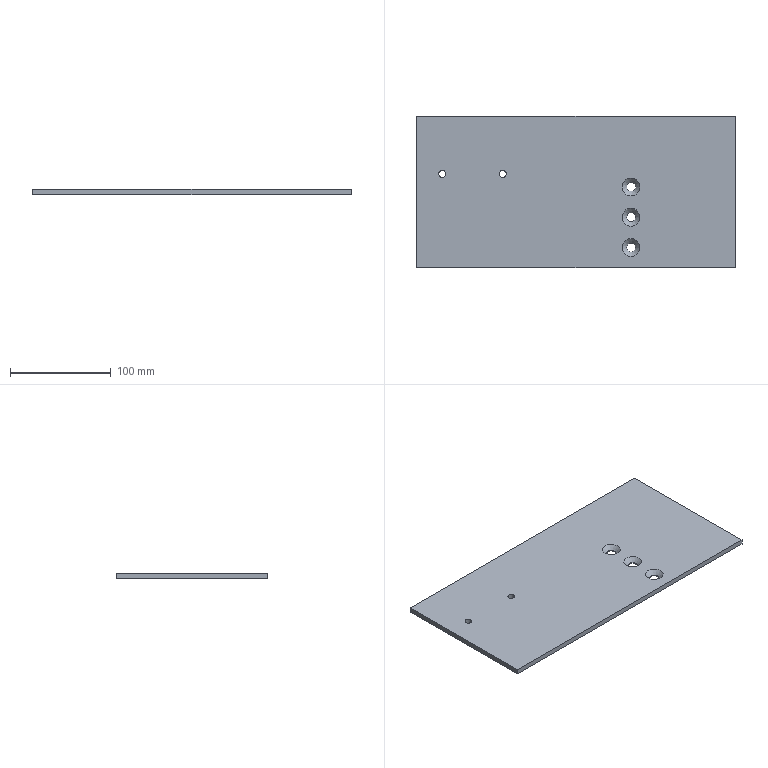Part | NX | features BREP 1 | 1 solid | 14 faces | box 315 x 150 x 5 mm | volume 233899 mm3 | plane 6 | cylinder 5 | cone 3 | commonest cylinder face diameters 9 x3 6.8 x2
STEP:
#1=CARTESIAN_POINT('',(-129.1,18.,5.));
#2=VERTEX_POINT('',#1);
#3=CARTESIAN_POINT('',(-132.5,18.,5.));
#4=DIRECTION('',(0.,0.,1.));
#5=DIRECTION('',(1.,0.,0.));
#6=AXIS2_PLACEMENT_3D('',#3,#4,#5);
#7=CIRCLE('',#6,3.4);
#8=EDGE_CURVE('',#2,#2,#7,.T.);
#9=ORIENTED_EDGE('',*,*,#8,.T.);
#10=EDGE_LOOP('',(#9));
#11=FACE_BOUND('',#10,.T.);
#12=CARTESIAN_POINT('',(-129.1,18.,0.));
#13=VERTEX_POINT('',#12);
#14=CARTESIAN_POINT('',(-132.5,18.,0.));
#15=DIRECTION('',(0.,0.,1.));
#16=DIRECTION('',(1.,0.,0.));
#17=AXIS2_PLACEMENT_3D('',#14,#15,#16);
#18=CIRCLE('',#17,3.4);
#19=EDGE_CURVE('',#13,#13,#18,.T.);
#20=ORIENTED_EDGE('',*,*,#19,.F.);
#21=EDGE_LOOP('',(#20));
#22=FACE_BOUND('',#21,.T.);
#23=CARTESIAN_POINT('',(-132.5,18.,5.));
#24=DIRECTION('',(0.,0.,1.));
#25=DIRECTION('',(1.,0.,0.));
#26=AXIS2_PLACEMENT_3D('',#23,#24,#25);
#27=CYLINDRICAL_SURFACE('',#26,3.4);
#28=ADVANCED_FACE('',(#11,#22),#27,.F.);
#29=CARTESIAN_POINT('',(-69.1,18.,5.));
#30=VERTEX_POINT('',#29);
#31=CARTESIAN_POINT('',(-72.5,18.,5.));
#32=DIRECTION('',(0.,0.,1.));
#33=DIRECTION('',(1.,0.,0.));
#34=AXIS2_PLACEMENT_3D('',#31,#32,#33);
#35=CIRCLE('',#34,3.4);
#36=EDGE_CURVE('',#30,#30,#35,.T.);
#37=ORIENTED_EDGE('',*,*,#36,.T.);
#38=EDGE_LOOP('',(#37));
#39=FACE_BOUND('',#38,.T.);
#40=CARTESIAN_POINT('',(-69.1,18.,0.));
#41=VERTEX_POINT('',#40);
#42=CARTESIAN_POINT('',(-72.5,18.,0.));
#43=DIRECTION('',(0.,0.,1.));
#44=DIRECTION('',(1.,0.,0.));
#45=AXIS2_PLACEMENT_3D('',#42,#43,#44);
#46=CIRCLE('',#45,3.4);
#47=EDGE_CURVE('',#41,#41,#46,.T.);
#48=ORIENTED_EDGE('',*,*,#47,.F.);
#49=EDGE_LOOP('',(#48));
#50=FACE_BOUND('',#49,.T.);
#51=CARTESIAN_POINT('',(-72.5,18.,5.));
#52=DIRECTION('',(0.,0.,1.));
#53=DIRECTION('',(1.,0.,0.));
#54=AXIS2_PLACEMENT_3D('',#51,#52,#53);
#55=CYLINDRICAL_SURFACE('',#54,3.4);
#56=ADVANCED_FACE('',(#39,#50),#55,.F.);
#57=CARTESIAN_POINT('',(63.3,-55.,5.));
#58=VERTEX_POINT('',#57);
#59=CARTESIAN_POINT('',(54.5,-55.,5.));
#60=DIRECTION('',(0.,0.,1.));
#61=DIRECTION('',(1.,0.,0.));
#62=AXIS2_PLACEMENT_3D('',#59,#60,#61);
#63=CIRCLE('',#62,8.8);
#64=EDGE_CURVE('',#58,#58,#63,.T.);
#65=ORIENTED_EDGE('',*,*,#64,.T.);
#66=EDGE_LOOP('',(#65));
#67=FACE_BOUND('',#66,.T.);
#68=CARTESIAN_POINT('',(59.,-55.,0.7));
#69=VERTEX_POINT('',#68);
#70=CARTESIAN_POINT('',(54.5,-55.,0.7));
#71=DIRECTION('',(0.,0.,1.));
#72=DIRECTION('',(1.,0.,0.));
#73=AXIS2_PLACEMENT_3D('',#70,#71,#72);
#74=CIRCLE('',#73,4.5);
#75=EDGE_CURVE('',#69,#69,#74,.T.);
#76=ORIENTED_EDGE('',*,*,#75,.F.);
#77=EDGE_LOOP('',(#76));
#78=FACE_BOUND('',#77,.T.);
#79=CARTESIAN_POINT('',(54.5,-55.,5.));
#80=DIRECTION('',(0.,0.,1.));
#81=DIRECTION('',(1.,0.,0.));
#82=AXIS2_PLACEMENT_3D('',#79,#80,#81);
#83=CONICAL_SURFACE('',#82,8.8,0.7854);
#84=ADVANCED_FACE('',(#67,#78),#83,.F.);
#85=ORIENTED_EDGE('',*,*,#75,.T.);
#86=EDGE_LOOP('',(#85));
#87=FACE_BOUND('',#86,.T.);
#88=CARTESIAN_POINT('',(59.,-55.,0.));
#89=VERTEX_POINT('',#88);
#90=CARTESIAN_POINT('',(54.5,-55.,0.));
#91=DIRECTION('',(0.,0.,1.));
#92=DIRECTION('',(1.,0.,0.));
#93=AXIS2_PLACEMENT_3D('',#90,#91,#92);
#94=CIRCLE('',#93,4.5);
#95=EDGE_CURVE('',#89,#89,#94,.T.);
#96=ORIENTED_EDGE('',*,*,#95,.F.);
#97=EDGE_LOOP('',(#96));
#98=FACE_BOUND('',#97,.T.);
#99=CARTESIAN_POINT('',(54.5,-55.,5.));
#100=DIRECTION('',(0.,0.,1.));
#101=DIRECTION('',(1.,0.,0.));
#102=AXIS2_PLACEMENT_3D('',#99,#100,#101);
#103=CYLINDRICAL_SURFACE('',#102,4.5);
#104=ADVANCED_FACE('',(#87,#98),#103,.F.);
#105=CARTESIAN_POINT('',(63.3,-25.,5.));
#106=VERTEX_POINT('',#105);
#107=CARTESIAN_POINT('',(54.5,-25.,5.));
#108=DIRECTION('',(0.,0.,1.));
#109=DIRECTION('',(1.,0.,0.));
#110=AXIS2_PLACEMENT_3D('',#107,#108,#109);
#111=CIRCLE('',#110,8.8);
#112=EDGE_CURVE('',#106,#106,#111,.T.);
#113=ORIENTED_EDGE('',*,*,#112,.T.);
#114=EDGE_LOOP('',(#113));
#115=FACE_BOUND('',#114,.T.);
#116=CARTESIAN_POINT('',(59.,-25.,0.7));
#117=VERTEX_POINT('',#116);
#118=CARTESIAN_POINT('',(54.5,-25.,0.7));
#119=DIRECTION('',(0.,0.,1.));
#120=DIRECTION('',(1.,0.,0.));
#121=AXIS2_PLACEMENT_3D('',#118,#119,#120);
#122=CIRCLE('',#121,4.5);
#123=EDGE_CURVE('',#117,#117,#122,.T.);
#124=ORIENTED_EDGE('',*,*,#123,.F.);
#125=EDGE_LOOP('',(#124));
#126=FACE_BOUND('',#125,.T.);
#127=CARTESIAN_POINT('',(54.5,-25.,5.));
#128=DIRECTION('',(0.,0.,1.));
#129=DIRECTION('',(1.,0.,0.));
#130=AXIS2_PLACEMENT_3D('',#127,#128,#129);
#131=CONICAL_SURFACE('',#130,8.8,0.7854);
#132=ADVANCED_FACE('',(#115,#126),#131,.F.);
#133=ORIENTED_EDGE('',*,*,#123,.T.);
#134=EDGE_LOOP('',(#133));
#135=FACE_BOUND('',#134,.T.);
#136=CARTESIAN_POINT('',(59.,-25.,0.));
#137=VERTEX_POINT('',#136);
#138=CARTESIAN_POINT('',(54.5,-25.,0.));
#139=DIRECTION('',(0.,0.,1.));
#140=DIRECTION('',(1.,0.,0.));
#141=AXIS2_PLACEMENT_3D('',#138,#139,#140);
#142=CIRCLE('',#141,4.5);
#143=EDGE_CURVE('',#137,#137,#142,.T.);
#144=ORIENTED_EDGE('',*,*,#143,.F.);
#145=EDGE_LOOP('',(#144));
#146=FACE_BOUND('',#145,.T.);
#147=CARTESIAN_POINT('',(54.5,-25.,5.));
#148=DIRECTION('',(0.,0.,1.));
#149=DIRECTION('',(1.,0.,0.));
#150=AXIS2_PLACEMENT_3D('',#147,#148,#149);
#151=CYLINDRICAL_SURFACE('',#150,4.5);
#152=ADVANCED_FACE('',(#135,#146),#151,.F.);
#153=CARTESIAN_POINT('',(63.3,5.,5.));
#154=VERTEX_POINT('',#153);
#155=CARTESIAN_POINT('',(54.5,5.,5.));
#156=DIRECTION('',(0.,0.,1.));
#157=DIRECTION('',(1.,0.,0.));
#158=AXIS2_PLACEMENT_3D('',#155,#156,#157);
#159=CIRCLE('',#158,8.8);
#160=EDGE_CURVE('',#154,#154,#159,.T.);
#161=ORIENTED_EDGE('',*,*,#160,.T.);
#162=EDGE_LOOP('',(#161));
#163=FACE_BOUND('',#162,.T.);
#164=CARTESIAN_POINT('',(59.,5.,0.7));
#165=VERTEX_POINT('',#164);
#166=CARTESIAN_POINT('',(54.5,5.,0.7));
#167=DIRECTION('',(0.,0.,1.));
#168=DIRECTION('',(1.,0.,0.));
#169=AXIS2_PLACEMENT_3D('',#166,#167,#168);
#170=CIRCLE('',#169,4.5);
#171=EDGE_CURVE('',#165,#165,#170,.T.);
#172=ORIENTED_EDGE('',*,*,#171,.F.);
#173=EDGE_LOOP('',(#172));
#174=FACE_BOUND('',#173,.T.);
#175=CARTESIAN_POINT('',(54.5,5.,5.));
#176=DIRECTION('',(0.,0.,1.));
#177=DIRECTION('',(1.,0.,0.));
#178=AXIS2_PLACEMENT_3D('',#175,#176,#177);
#179=CONICAL_SURFACE('',#178,8.8,0.7854);
#180=ADVANCED_FACE('',(#163,#174),#179,.F.);
#181=ORIENTED_EDGE('',*,*,#171,.T.);
#182=EDGE_LOOP('',(#181));
#183=FACE_BOUND('',#182,.T.);
#184=CARTESIAN_POINT('',(59.,5.,0.));
#185=VERTEX_POINT('',#184);
#186=CARTESIAN_POINT('',(54.5,5.,0.));
#187=DIRECTION('',(0.,0.,1.));
#188=DIRECTION('',(1.,0.,0.));
#189=AXIS2_PLACEMENT_3D('',#186,#187,#188);
#190=CIRCLE('',#189,4.5);
#191=EDGE_CURVE('',#185,#185,#190,.T.);
#192=ORIENTED_EDGE('',*,*,#191,.F.);
#193=EDGE_LOOP('',(#192));
#194=FACE_BOUND('',#193,.T.);
#195=CARTESIAN_POINT('',(54.5,5.,5.));
#196=DIRECTION('',(0.,0.,1.));
#197=DIRECTION('',(1.,0.,0.));
#198=AXIS2_PLACEMENT_3D('',#195,#196,#197);
#199=CYLINDRICAL_SURFACE('',#198,4.5);
#200=ADVANCED_FACE('',(#183,#194),#199,.F.);
#201=CARTESIAN_POINT('',(157.5,-75.,0.));
#202=VERTEX_POINT('',#201);
#203=CARTESIAN_POINT('',(157.5,75.,0.));
#204=VERTEX_POINT('',#203);
#205=CARTESIAN_POINT('',(157.5,-75.,0.));
#206=DIRECTION('',(0.,1.,0.));
#207=VECTOR('',#206,1000.);
#208=LINE('',#205,#207);
#209=EDGE_CURVE('',#202,#204,#208,.T.);
#210=ORIENTED_EDGE('',*,*,#209,.T.);
#211=CARTESIAN_POINT('',(157.5,75.,5.));
#212=VERTEX_POINT('',#211);
#213=CARTESIAN_POINT('',(157.5,75.,5.));
#214=DIRECTION('',(0.,0.,-1.));
#215=VECTOR('',#214,1000.);
#216=LINE('',#213,#215);
#217=EDGE_CURVE('',#212,#204,#216,.T.);
#218=ORIENTED_EDGE('',*,*,#217,.F.);
#219=CARTESIAN_POINT('',(157.5,-75.,5.));
#220=VERTEX_POINT('',#219);
#221=CARTESIAN_POINT('',(157.5,-75.,5.));
#222=DIRECTION('',(0.,1.,0.));
#223=VECTOR('',#222,1000.);
#224=LINE('',#221,#223);
#225=EDGE_CURVE('',#220,#212,#224,.T.);
#226=ORIENTED_EDGE('',*,*,#225,.F.);
#227=CARTESIAN_POINT('',(157.5,-75.,5.));
#228=DIRECTION('',(0.,0.,-1.));
#229=VECTOR('',#228,1000.);
#230=LINE('',#227,#229);
#231=EDGE_CURVE('',#220,#202,#230,.T.);
#232=ORIENTED_EDGE('',*,*,#231,.T.);
#233=EDGE_LOOP('',(#210,#218,#226,#232));
#234=FACE_BOUND('',#233,.T.);
#235=CARTESIAN_POINT('',(157.5,-75.,5.));
#236=DIRECTION('',(-1.,0.,0.));
#237=DIRECTION('',(0.,0.,1.));
#238=AXIS2_PLACEMENT_3D('',#235,#236,#237);
#239=PLANE('',#238);
#240=ADVANCED_FACE('',(#234),#239,.F.);
#241=CARTESIAN_POINT('',(-157.5,75.,0.));
#242=VERTEX_POINT('',#241);
#243=CARTESIAN_POINT('',(-157.5,75.,0.));
#244=DIRECTION('',(-1.,0.,0.));
#245=VECTOR('',#244,1000.);
#246=LINE('',#243,#245);
#247=EDGE_CURVE('',#204,#242,#246,.T.);
#248=ORIENTED_EDGE('',*,*,#247,.T.);
#249=CARTESIAN_POINT('',(-157.5,75.,5.));
#250=VERTEX_POINT('',#249);
#251=CARTESIAN_POINT('',(-157.5,75.,5.));
#252=DIRECTION('',(0.,0.,-1.));
#253=VECTOR('',#252,1000.);
#254=LINE('',#251,#253);
#255=EDGE_CURVE('',#250,#242,#254,.T.);
#256=ORIENTED_EDGE('',*,*,#255,.F.);
#257=CARTESIAN_POINT('',(-157.5,75.,5.));
#258=DIRECTION('',(-1.,0.,0.));
#259=VECTOR('',#258,1000.);
#260=LINE('',#257,#259);
#261=EDGE_CURVE('',#212,#250,#260,.T.);
#262=ORIENTED_EDGE('',*,*,#261,.F.);
#263=ORIENTED_EDGE('',*,*,#217,.T.);
#264=EDGE_LOOP('',(#248,#256,#262,#263));
#265=FACE_BOUND('',#264,.T.);
#266=CARTESIAN_POINT('',(-157.5,75.,5.));
#267=DIRECTION('',(0.,-1.,0.));
#268=DIRECTION('',(0.,0.,-1.));
#269=AXIS2_PLACEMENT_3D('',#266,#267,#268);
#270=PLANE('',#269);
#271=ADVANCED_FACE('',(#265),#270,.F.);
#272=CARTESIAN_POINT('',(-157.5,-75.,0.));
#273=VERTEX_POINT('',#272);
#274=CARTESIAN_POINT('',(-157.5,-75.,0.));
#275=DIRECTION('',(0.,-1.,0.));
#276=VECTOR('',#275,1000.);
#277=LINE('',#274,#276);
#278=EDGE_CURVE('',#242,#273,#277,.T.);
#279=ORIENTED_EDGE('',*,*,#278,.T.);
#280=CARTESIAN_POINT('',(-157.5,-75.,5.));
#281=VERTEX_POINT('',#280);
#282=CARTESIAN_POINT('',(-157.5,-75.,5.));
#283=DIRECTION('',(0.,0.,-1.));
#284=VECTOR('',#283,1000.);
#285=LINE('',#282,#284);
#286=EDGE_CURVE('',#281,#273,#285,.T.);
#287=ORIENTED_EDGE('',*,*,#286,.F.);
#288=CARTESIAN_POINT('',(-157.5,-75.,5.));
#289=DIRECTION('',(0.,-1.,0.));
#290=VECTOR('',#289,1000.);
#291=LINE('',#288,#290);
#292=EDGE_CURVE('',#250,#281,#291,.T.);
#293=ORIENTED_EDGE('',*,*,#292,.F.);
#294=ORIENTED_EDGE('',*,*,#255,.T.);
#295=EDGE_LOOP('',(#279,#287,#293,#294));
#296=FACE_BOUND('',#295,.T.);
#297=CARTESIAN_POINT('',(-157.5,-75.,5.));
#298=DIRECTION('',(1.,0.,0.));
#299=DIRECTION('',(0.,0.,-1.));
#300=AXIS2_PLACEMENT_3D('',#297,#298,#299);
#301=PLANE('',#300);
#302=ADVANCED_FACE('',(#296),#301,.F.);
#303=CARTESIAN_POINT('',(-157.5,-75.,0.));
#304=DIRECTION('',(1.,0.,0.));
#305=VECTOR('',#304,1000.);
#306=LINE('',#303,#305);
#307=EDGE_CURVE('',#273,#202,#306,.T.);
#308=ORIENTED_EDGE('',*,*,#307,.T.);
#309=ORIENTED_EDGE('',*,*,#231,.F.);
#310=CARTESIAN_POINT('',(-157.5,-75.,5.));
#311=DIRECTION('',(1.,0.,0.));
#312=VECTOR('',#311,1000.);
#313=LINE('',#310,#312);
#314=EDGE_CURVE('',#281,#220,#313,.T.);
#315=ORIENTED_EDGE('',*,*,#314,.F.);
#316=ORIENTED_EDGE('',*,*,#286,.T.);
#317=EDGE_LOOP('',(#308,#309,#315,#316));
#318=FACE_BOUND('',#317,.T.);
#319=CARTESIAN_POINT('',(-157.5,-75.,5.));
#320=DIRECTION('',(0.,1.,0.));
#321=DIRECTION('',(0.,0.,1.));
#322=AXIS2_PLACEMENT_3D('',#319,#320,#321);
#323=PLANE('',#322);
#324=ADVANCED_FACE('',(#318),#323,.F.);
#325=ORIENTED_EDGE('',*,*,#8,.F.);
#326=EDGE_LOOP('',(#325));
#327=FACE_BOUND('',#326,.T.);
#328=ORIENTED_EDGE('',*,*,#36,.F.);
#329=EDGE_LOOP('',(#328));
#330=FACE_BOUND('',#329,.T.);
#331=ORIENTED_EDGE('',*,*,#64,.F.);
#332=EDGE_LOOP('',(#331));
#333=FACE_BOUND('',#332,.T.);
#334=ORIENTED_EDGE('',*,*,#112,.F.);
#335=EDGE_LOOP('',(#334));
#336=FACE_BOUND('',#335,.T.);
#337=ORIENTED_EDGE('',*,*,#160,.F.);
#338=EDGE_LOOP('',(#337));
#339=FACE_BOUND('',#338,.T.);
#340=ORIENTED_EDGE('',*,*,#225,.T.);
#341=ORIENTED_EDGE('',*,*,#261,.T.);
#342=ORIENTED_EDGE('',*,*,#292,.T.);
#343=ORIENTED_EDGE('',*,*,#314,.T.);
#344=EDGE_LOOP('',(#340,#341,#342,#343));
#345=FACE_BOUND('',#344,.T.);
#346=CARTESIAN_POINT('',(0.,0.,5.));
#347=DIRECTION('',(0.,0.,-1.));
#348=DIRECTION('',(-1.,0.,0.));
#349=AXIS2_PLACEMENT_3D('',#346,#347,#348);
#350=PLANE('',#349);
#351=ADVANCED_FACE('',(#327,#330,#333,#336,#339,#345),#350,.F.);
#352=ORIENTED_EDGE('',*,*,#19,.T.);
#353=EDGE_LOOP('',(#352));
#354=FACE_BOUND('',#353,.T.);
#355=ORIENTED_EDGE('',*,*,#47,.T.);
#356=EDGE_LOOP('',(#355));
#357=FACE_BOUND('',#356,.T.);
#358=ORIENTED_EDGE('',*,*,#95,.T.);
#359=EDGE_LOOP('',(#358));
#360=FACE_BOUND('',#359,.T.);
#361=ORIENTED_EDGE('',*,*,#143,.T.);
#362=EDGE_LOOP('',(#361));
#363=FACE_BOUND('',#362,.T.);
#364=ORIENTED_EDGE('',*,*,#191,.T.);
#365=EDGE_LOOP('',(#364));
#366=FACE_BOUND('',#365,.T.);
#367=ORIENTED_EDGE('',*,*,#209,.F.);
#368=ORIENTED_EDGE('',*,*,#307,.F.);
#369=ORIENTED_EDGE('',*,*,#278,.F.);
#370=ORIENTED_EDGE('',*,*,#247,.F.);
#371=EDGE_LOOP('',(#367,#368,#369,#370));
#372=FACE_BOUND('',#371,.T.);
#373=CARTESIAN_POINT('',(0.,0.,0.));
#374=DIRECTION('',(0.,0.,-1.));
#375=DIRECTION('',(-1.,0.,0.));
#376=AXIS2_PLACEMENT_3D('',#373,#374,#375);
#377=PLANE('',#376);
#378=ADVANCED_FACE('',(#354,#357,#360,#363,#366,#372),#377,.T.);
#379=CLOSED_SHELL('',(#28,#56,#84,#104,#132,#152,#180,#200,#240,#271,#302,#324,#351,#378));
#380=MANIFOLD_SOLID_BREP('',#379);
#381=(LENGTH_UNIT()NAMED_UNIT(*)SI_UNIT(.MILLI.,.METRE.));
#382=UNCERTAINTY_MEASURE_WITH_UNIT(LENGTH_MEASURE(0.00001),#381,'','');
#383=(NAMED_UNIT(*)PLANE_ANGLE_UNIT()SI_UNIT($,.RADIAN.));
#384=(NAMED_UNIT(*)SI_UNIT($,.STERADIAN.)SOLID_ANGLE_UNIT());
#385=(GEOMETRIC_REPRESENTATION_CONTEXT(3)GLOBAL_UNCERTAINTY_ASSIGNED_CONTEXT((#382))GLOBAL_UNIT_ASSIGNED_CONTEXT((#381,#383,#384))REPRESENTATION_CONTEXT('',''));
#386=ADVANCED_BREP_SHAPE_REPRESENTATION('',(#380),#385);